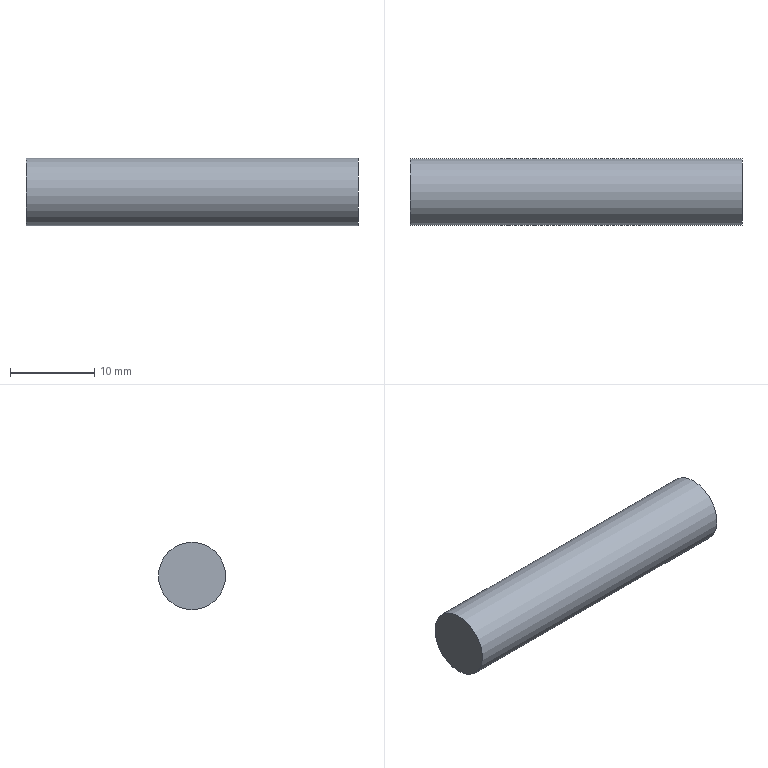Part | STEP file | solid 92 | 1 solid | 3 faces | box 39.5 x 8 x 8 mm | volume 1985 mm3 | plane 2 | cylinder 1 | commonest cylinder face diameters 8 x1